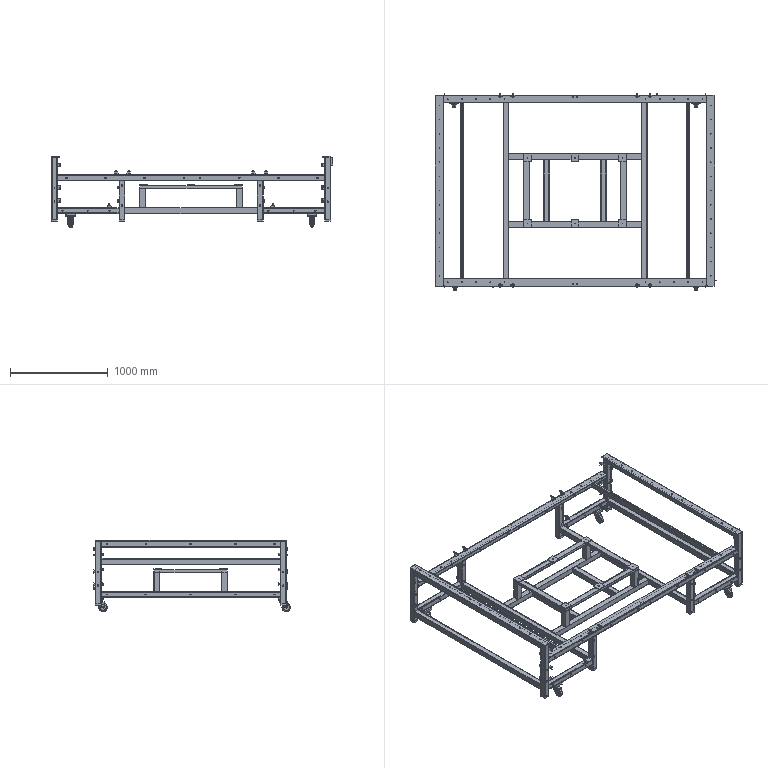Part | SolidWorks | features BaseBody 135 | 135 solids | 3210 faces | volume 30695338 mm3 | plane 1580 | cylinder 1430 | cone 120 | torus 56 | spline 24 | commonest cylinder face diameters 7 x496 6 x176 12 x136 4 x134 6.8 x124 5 x76